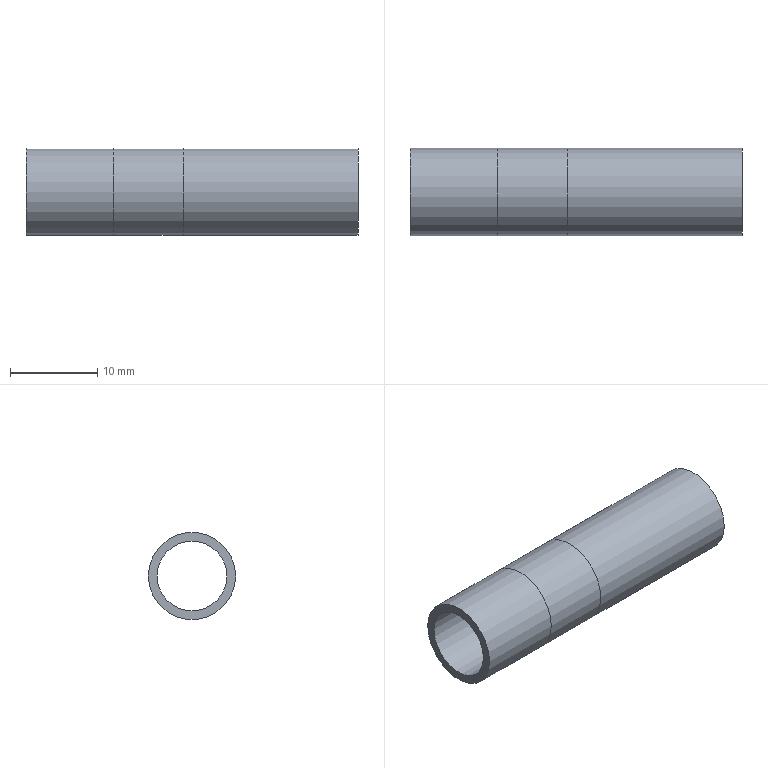Part | STEP file | 1-12.2 | 1 solid | 6 faces | box 38 x 10 x 10 mm | volume 1074 mm3 | cylinder 4 | plane 2 | commonest cylinder face diameters 10 x3 8 x1
STEP:
#1=CARTESIAN_POINT('',(0.,0.,0.));
#2=DIRECTION('',(0.,0.,1.));
#3=DIRECTION('',(1.,0.,0.));
#4=AXIS2_PLACEMENT_3D('',#1,#2,#3);
#5=CARTESIAN_POINT('',(-19.,5.,0.));
#6=VERTEX_POINT('',#5);
#7=CARTESIAN_POINT('',(-19.,0.,0.));
#8=DIRECTION('',(1.,0.,0.));
#9=DIRECTION('',(0.,1.,0.));
#10=AXIS2_PLACEMENT_3D('',#7,#8,#9);
#11=CIRCLE('',#10,5.);
#12=CARTESIAN_POINT('',(-19.,-1.34,0.));
#13=DIRECTION('',(1.,0.,0.));
#14=DIRECTION('',(0.,1.,0.));
#15=AXIS2_PLACEMENT_3D('',#12,#13,#14);
#16=PLANE('',#15);
#17=CARTESIAN_POINT('',(1.34,0.));
#18=DIRECTION('',(1.,0.));
#19=AXIS2_PLACEMENT_2D('',#17,#18);
#20=CIRCLE('',#19,5.);
#21=(GEOMETRIC_REPRESENTATION_CONTEXT(2)PARAMETRIC_REPRESENTATION_CONTEXT()REPRESENTATION_CONTEXT('',''));
#22=DEFINITIONAL_REPRESENTATION('',(#20),#21);
#23=PCURVE('',#16,#22);
#24=CARTESIAN_POINT('',(-19.,0.,0.));
#25=DIRECTION('',(1.,0.,0.));
#26=DIRECTION('',(0.,1.,0.));
#27=AXIS2_PLACEMENT_3D('',#24,#25,#26);
#28=CYLINDRICAL_SURFACE('',#27,5.);
#29=CARTESIAN_POINT('',(0.,0.));
#30=DIRECTION('',(1.,0.));
#31=VECTOR('',#30,1.);
#32=LINE('',#29,#31);
#33=(GEOMETRIC_REPRESENTATION_CONTEXT(2)PARAMETRIC_REPRESENTATION_CONTEXT()REPRESENTATION_CONTEXT('',''));
#34=DEFINITIONAL_REPRESENTATION('',(#32),#33);
#35=PCURVE('',#28,#34);
#36=SURFACE_CURVE('',#11,(#23,#35),.PCURVE_S1.);
#37=EDGE_CURVE('',#6,#6,#36,.T.);
#38=ORIENTED_EDGE('',*,*,#37,.T.);
#39=EDGE_LOOP('',(#38));
#40=FACE_BOUND('',#39,.F.);
#41=CARTESIAN_POINT('',(-19.,4.,0.));
#42=VERTEX_POINT('',#41);
#43=CARTESIAN_POINT('',(-19.,0.,0.));
#44=DIRECTION('',(-1.,0.,0.));
#45=DIRECTION('',(0.,1.,0.));
#46=AXIS2_PLACEMENT_3D('',#43,#44,#45);
#47=CIRCLE('',#46,4.);
#48=CARTESIAN_POINT('',(5.34,0.));
#49=CARTESIAN_POINT('',(5.34,-6.928));
#50=CARTESIAN_POINT('',(-0.6603,-3.464));
#51=CARTESIAN_POINT('',(-6.66,0.));
#52=CARTESIAN_POINT('',(-0.6603,3.464));
#53=CARTESIAN_POINT('',(5.34,6.928));
#54=CARTESIAN_POINT('',(5.34,0.));
#55=(BOUNDED_CURVE()B_SPLINE_CURVE(2,(#48,#49,#50,#51,#52,#53,#54),.UNSPECIFIED.,.T.,.F.)B_SPLINE_CURVE_WITH_KNOTS((1,2,2,2,2,1),(-2.094,0.,2.094,4.189,6.283,8.378),.UNSPECIFIED.)CURVE()GEOMETRIC_REPRESENTATION_ITEM()RATIONAL_B_SPLINE_CURVE((1.,0.5,1.,0.5,1.,0.5,1.))REPRESENTATION_ITEM(''));
#56=(GEOMETRIC_REPRESENTATION_CONTEXT(2)PARAMETRIC_REPRESENTATION_CONTEXT()REPRESENTATION_CONTEXT('',''));
#57=DEFINITIONAL_REPRESENTATION('',(#55),#56);
#58=PCURVE('',#16,#57);
#59=CARTESIAN_POINT('',(-19.,0.,0.));
#60=DIRECTION('',(1.,0.,0.));
#61=DIRECTION('',(0.,1.,0.));
#62=AXIS2_PLACEMENT_3D('',#59,#60,#61);
#63=CYLINDRICAL_SURFACE('',#62,4.);
#64=CARTESIAN_POINT('',(6.283,0.));
#65=DIRECTION('',(-1.,0.));
#66=VECTOR('',#65,1.);
#67=LINE('',#64,#66);
#68=(GEOMETRIC_REPRESENTATION_CONTEXT(2)PARAMETRIC_REPRESENTATION_CONTEXT()REPRESENTATION_CONTEXT('',''));
#69=DEFINITIONAL_REPRESENTATION('',(#67),#68);
#70=PCURVE('',#63,#69);
#71=SURFACE_CURVE('',#47,(#58,#70),.PCURVE_S1.);
#72=EDGE_CURVE('',#42,#42,#71,.T.);
#73=ORIENTED_EDGE('',*,*,#72,.T.);
#74=EDGE_LOOP('',(#73));
#75=FACE_BOUND('',#74,.F.);
#76=ADVANCED_FACE('',(#40,#75),#16,.F.);
#77=CARTESIAN_POINT('',(19.,5.,0.));
#78=VERTEX_POINT('',#77);
#79=CARTESIAN_POINT('',(19.,0.,0.));
#80=DIRECTION('',(1.,0.,0.));
#81=DIRECTION('',(0.,1.,0.));
#82=AXIS2_PLACEMENT_3D('',#79,#80,#81);
#83=CIRCLE('',#82,5.);
#84=CARTESIAN_POINT('',(19.,-1.34,0.));
#85=DIRECTION('',(1.,0.,0.));
#86=DIRECTION('',(0.,1.,0.));
#87=AXIS2_PLACEMENT_3D('',#84,#85,#86);
#88=PLANE('',#87);
#89=CARTESIAN_POINT('',(1.34,0.));
#90=DIRECTION('',(1.,0.));
#91=AXIS2_PLACEMENT_2D('',#89,#90);
#92=CIRCLE('',#91,5.);
#93=(GEOMETRIC_REPRESENTATION_CONTEXT(2)PARAMETRIC_REPRESENTATION_CONTEXT()REPRESENTATION_CONTEXT('',''));
#94=DEFINITIONAL_REPRESENTATION('',(#92),#93);
#95=PCURVE('',#88,#94);
#96=CARTESIAN_POINT('',(-1.,0.,0.));
#97=DIRECTION('',(1.,0.,0.));
#98=DIRECTION('',(0.,1.,0.));
#99=AXIS2_PLACEMENT_3D('',#96,#97,#98);
#100=CYLINDRICAL_SURFACE('',#99,5.);
#101=CARTESIAN_POINT('',(0.,20.));
#102=DIRECTION('',(1.,0.));
#103=VECTOR('',#102,1.);
#104=LINE('',#101,#103);
#105=(GEOMETRIC_REPRESENTATION_CONTEXT(2)PARAMETRIC_REPRESENTATION_CONTEXT()REPRESENTATION_CONTEXT('',''));
#106=DEFINITIONAL_REPRESENTATION('',(#104),#105);
#107=PCURVE('',#100,#106);
#108=SURFACE_CURVE('',#83,(#95,#107),.PCURVE_S1.);
#109=EDGE_CURVE('',#78,#78,#108,.T.);
#110=ORIENTED_EDGE('',*,*,#109,.T.);
#111=EDGE_LOOP('',(#110));
#112=FACE_BOUND('',#111,.T.);
#113=CARTESIAN_POINT('',(19.,4.,0.));
#114=VERTEX_POINT('',#113);
#115=CARTESIAN_POINT('',(19.,0.,0.));
#116=DIRECTION('',(-1.,0.,0.));
#117=DIRECTION('',(0.,1.,0.));
#118=AXIS2_PLACEMENT_3D('',#115,#116,#117);
#119=CIRCLE('',#118,4.);
#120=CARTESIAN_POINT('',(5.34,0.));
#121=CARTESIAN_POINT('',(5.34,-6.928));
#122=CARTESIAN_POINT('',(-0.6603,-3.464));
#123=CARTESIAN_POINT('',(-6.66,0.));
#124=CARTESIAN_POINT('',(-0.6603,3.464));
#125=CARTESIAN_POINT('',(5.34,6.928));
#126=CARTESIAN_POINT('',(5.34,0.));
#127=(BOUNDED_CURVE()B_SPLINE_CURVE(2,(#120,#121,#122,#123,#124,#125,#126),.UNSPECIFIED.,.T.,.F.)B_SPLINE_CURVE_WITH_KNOTS((1,2,2,2,2,1),(-2.094,0.,2.094,4.189,6.283,8.378),.UNSPECIFIED.)CURVE()GEOMETRIC_REPRESENTATION_ITEM()RATIONAL_B_SPLINE_CURVE((1.,0.5,1.,0.5,1.,0.5,1.))REPRESENTATION_ITEM(''));
#128=(GEOMETRIC_REPRESENTATION_CONTEXT(2)PARAMETRIC_REPRESENTATION_CONTEXT()REPRESENTATION_CONTEXT('',''));
#129=DEFINITIONAL_REPRESENTATION('',(#127),#128);
#130=PCURVE('',#88,#129);
#131=CARTESIAN_POINT('',(6.283,38.));
#132=DIRECTION('',(-1.,0.));
#133=VECTOR('',#132,1.);
#134=LINE('',#131,#133);
#135=(GEOMETRIC_REPRESENTATION_CONTEXT(2)PARAMETRIC_REPRESENTATION_CONTEXT()REPRESENTATION_CONTEXT('',''));
#136=DEFINITIONAL_REPRESENTATION('',(#134),#135);
#137=PCURVE('',#63,#136);
#138=SURFACE_CURVE('',#119,(#130,#137),.PCURVE_S1.);
#139=EDGE_CURVE('',#114,#114,#138,.T.);
#140=ORIENTED_EDGE('',*,*,#139,.T.);
#141=EDGE_LOOP('',(#140));
#142=FACE_BOUND('',#141,.T.);
#143=ADVANCED_FACE('',(#112,#142),#88,.T.);
#144=CARTESIAN_POINT('',(-19.,4.,0.));
#145=DIRECTION('',(1.,0.,0.));
#146=VECTOR('',#145,1.);
#147=LINE('',#144,#146);
#148=CARTESIAN_POINT('',(6.283,0.));
#149=DIRECTION('',(0.,1.));
#150=VECTOR('',#149,1.);
#151=LINE('',#148,#150);
#152=(GEOMETRIC_REPRESENTATION_CONTEXT(2)PARAMETRIC_REPRESENTATION_CONTEXT()REPRESENTATION_CONTEXT('',''));
#153=DEFINITIONAL_REPRESENTATION('',(#151),#152);
#154=PCURVE('',#63,#153);
#155=CARTESIAN_POINT('',(0.,0.));
#156=DIRECTION('',(0.,1.));
#157=VECTOR('',#156,1.);
#158=LINE('',#155,#157);
#159=(GEOMETRIC_REPRESENTATION_CONTEXT(2)PARAMETRIC_REPRESENTATION_CONTEXT()REPRESENTATION_CONTEXT('',''));
#160=DEFINITIONAL_REPRESENTATION('',(#158),#159);
#161=PCURVE('',#63,#160);
#162=SEAM_CURVE('',#147,(#154,#161),.PCURVE_S1.);
#163=EDGE_CURVE('',#42,#114,#162,.T.);
#164=ORIENTED_EDGE('',*,*,#163,.T.);
#165=ORIENTED_EDGE('',*,*,#139,.T.);
#166=ORIENTED_EDGE('',*,*,#163,.F.);
#167=ORIENTED_EDGE('',*,*,#72,.F.);
#168=EDGE_LOOP('',(#164,#165,#166,#167));
#169=FACE_BOUND('',#168,.F.);
#170=ADVANCED_FACE('',(#169),#63,.F.);
#171=ORIENTED_EDGE('',*,*,#37,.T.);
#172=CARTESIAN_POINT('',(-9.,5.,0.));
#173=VERTEX_POINT('',#172);
#174=CARTESIAN_POINT('',(-19.,5.,0.));
#175=DIRECTION('',(1.,0.,0.));
#176=VECTOR('',#175,1.);
#177=LINE('',#174,#176);
#178=CARTESIAN_POINT('',(6.283,0.));
#179=DIRECTION('',(0.,1.));
#180=VECTOR('',#179,1.);
#181=LINE('',#178,#180);
#182=(GEOMETRIC_REPRESENTATION_CONTEXT(2)PARAMETRIC_REPRESENTATION_CONTEXT()REPRESENTATION_CONTEXT('',''));
#183=DEFINITIONAL_REPRESENTATION('',(#181),#182);
#184=PCURVE('',#28,#183);
#185=CARTESIAN_POINT('',(0.,0.));
#186=DIRECTION('',(0.,1.));
#187=VECTOR('',#186,1.);
#188=LINE('',#185,#187);
#189=(GEOMETRIC_REPRESENTATION_CONTEXT(2)PARAMETRIC_REPRESENTATION_CONTEXT()REPRESENTATION_CONTEXT('',''));
#190=DEFINITIONAL_REPRESENTATION('',(#188),#189);
#191=PCURVE('',#28,#190);
#192=SEAM_CURVE('',#177,(#184,#191),.PCURVE_S1.);
#193=EDGE_CURVE('',#6,#173,#192,.T.);
#194=ORIENTED_EDGE('',*,*,#193,.T.);
#195=CARTESIAN_POINT('',(-9.,0.,0.));
#196=DIRECTION('',(1.,0.,0.));
#197=DIRECTION('',(0.,1.,0.));
#198=AXIS2_PLACEMENT_3D('',#195,#196,#197);
#199=CIRCLE('',#198,5.);
#200=CARTESIAN_POINT('',(0.,10.));
#201=DIRECTION('',(1.,0.));
#202=VECTOR('',#201,1.);
#203=LINE('',#200,#202);
#204=(GEOMETRIC_REPRESENTATION_CONTEXT(2)PARAMETRIC_REPRESENTATION_CONTEXT()REPRESENTATION_CONTEXT('',''));
#205=DEFINITIONAL_REPRESENTATION('',(#203),#204);
#206=PCURVE('',#28,#205);
#207=CARTESIAN_POINT('',(-19.,0.,0.));
#208=DIRECTION('',(1.,0.,0.));
#209=DIRECTION('',(0.,1.,0.));
#210=AXIS2_PLACEMENT_3D('',#207,#208,#209);
#211=CYLINDRICAL_SURFACE('',#210,5.);
#212=CARTESIAN_POINT('',(0.,10.));
#213=DIRECTION('',(1.,0.));
#214=VECTOR('',#213,1.);
#215=LINE('',#212,#214);
#216=(GEOMETRIC_REPRESENTATION_CONTEXT(2)PARAMETRIC_REPRESENTATION_CONTEXT()REPRESENTATION_CONTEXT('',''));
#217=DEFINITIONAL_REPRESENTATION('',(#215),#216);
#218=PCURVE('',#211,#217);
#219=SURFACE_CURVE('',#199,(#206,#218),.PCURVE_S1.);
#220=EDGE_CURVE('',#173,#173,#219,.T.);
#221=ORIENTED_EDGE('',*,*,#220,.F.);
#222=ORIENTED_EDGE('',*,*,#193,.F.);
#223=EDGE_LOOP('',(#171,#194,#221,#222));
#224=FACE_BOUND('',#223,.T.);
#225=ADVANCED_FACE('',(#224),#28,.T.);
#226=ORIENTED_EDGE('',*,*,#220,.T.);
#227=CARTESIAN_POINT('',(-1.,5.,0.));
#228=VERTEX_POINT('',#227);
#229=CARTESIAN_POINT('',(-9.,5.,0.));
#230=DIRECTION('',(1.,0.,0.));
#231=VECTOR('',#230,1.);
#232=LINE('',#229,#231);
#233=CARTESIAN_POINT('',(6.283,10.));
#234=DIRECTION('',(0.,1.));
#235=VECTOR('',#234,1.);
#236=LINE('',#233,#235);
#237=(GEOMETRIC_REPRESENTATION_CONTEXT(2)PARAMETRIC_REPRESENTATION_CONTEXT()REPRESENTATION_CONTEXT('',''));
#238=DEFINITIONAL_REPRESENTATION('',(#236),#237);
#239=PCURVE('',#211,#238);
#240=CARTESIAN_POINT('',(0.,10.));
#241=DIRECTION('',(0.,1.));
#242=VECTOR('',#241,1.);
#243=LINE('',#240,#242);
#244=(GEOMETRIC_REPRESENTATION_CONTEXT(2)PARAMETRIC_REPRESENTATION_CONTEXT()REPRESENTATION_CONTEXT('',''));
#245=DEFINITIONAL_REPRESENTATION('',(#243),#244);
#246=PCURVE('',#211,#245);
#247=SEAM_CURVE('',#232,(#239,#246),.PCURVE_S1.);
#248=EDGE_CURVE('',#173,#228,#247,.T.);
#249=ORIENTED_EDGE('',*,*,#248,.T.);
#250=CARTESIAN_POINT('',(-1.,0.,0.));
#251=DIRECTION('',(1.,0.,0.));
#252=DIRECTION('',(0.,1.,0.));
#253=AXIS2_PLACEMENT_3D('',#250,#251,#252);
#254=CIRCLE('',#253,5.);
#255=CARTESIAN_POINT('',(0.,18.));
#256=DIRECTION('',(1.,0.));
#257=VECTOR('',#256,1.);
#258=LINE('',#255,#257);
#259=(GEOMETRIC_REPRESENTATION_CONTEXT(2)PARAMETRIC_REPRESENTATION_CONTEXT()REPRESENTATION_CONTEXT('',''));
#260=DEFINITIONAL_REPRESENTATION('',(#258),#259);
#261=PCURVE('',#211,#260);
#262=CARTESIAN_POINT('',(0.,0.));
#263=DIRECTION('',(1.,0.));
#264=VECTOR('',#263,1.);
#265=LINE('',#262,#264);
#266=(GEOMETRIC_REPRESENTATION_CONTEXT(2)PARAMETRIC_REPRESENTATION_CONTEXT()REPRESENTATION_CONTEXT('',''));
#267=DEFINITIONAL_REPRESENTATION('',(#265),#266);
#268=PCURVE('',#100,#267);
#269=SURFACE_CURVE('',#254,(#261,#268),.PCURVE_S1.);
#270=EDGE_CURVE('',#228,#228,#269,.T.);
#271=ORIENTED_EDGE('',*,*,#270,.F.);
#272=ORIENTED_EDGE('',*,*,#248,.F.);
#273=EDGE_LOOP('',(#226,#249,#271,#272));
#274=FACE_BOUND('',#273,.T.);
#275=ADVANCED_FACE('',(#274),#211,.T.);
#276=ORIENTED_EDGE('',*,*,#109,.F.);
#277=CARTESIAN_POINT('',(-1.,5.,0.));
#278=DIRECTION('',(1.,0.,0.));
#279=VECTOR('',#278,1.);
#280=LINE('',#277,#279);
#281=CARTESIAN_POINT('',(0.,0.));
#282=DIRECTION('',(0.,1.));
#283=VECTOR('',#282,1.);
#284=LINE('',#281,#283);
#285=(GEOMETRIC_REPRESENTATION_CONTEXT(2)PARAMETRIC_REPRESENTATION_CONTEXT()REPRESENTATION_CONTEXT('',''));
#286=DEFINITIONAL_REPRESENTATION('',(#284),#285);
#287=PCURVE('',#100,#286);
#288=CARTESIAN_POINT('',(6.283,0.));
#289=DIRECTION('',(0.,1.));
#290=VECTOR('',#289,1.);
#291=LINE('',#288,#290);
#292=(GEOMETRIC_REPRESENTATION_CONTEXT(2)PARAMETRIC_REPRESENTATION_CONTEXT()REPRESENTATION_CONTEXT('',''));
#293=DEFINITIONAL_REPRESENTATION('',(#291),#292);
#294=PCURVE('',#100,#293);
#295=SEAM_CURVE('',#280,(#287,#294),.PCURVE_S1.);
#296=EDGE_CURVE('',#228,#78,#295,.T.);
#297=ORIENTED_EDGE('',*,*,#296,.F.);
#298=ORIENTED_EDGE('',*,*,#270,.T.);
#299=ORIENTED_EDGE('',*,*,#296,.T.);
#300=EDGE_LOOP('',(#276,#297,#298,#299));
#301=FACE_BOUND('',#300,.T.);
#302=ADVANCED_FACE('',(#301),#100,.T.);
#303=CLOSED_SHELL('',(#76,#143,#170,#225,#275,#302));
#304=MANIFOLD_SOLID_BREP('',#303);
#305=(LENGTH_UNIT()NAMED_UNIT(*)SI_UNIT(.MILLI.,.METRE.));
#306=UNCERTAINTY_MEASURE_WITH_UNIT(LENGTH_MEASURE(0.0000001),#305,'','');
#307=(NAMED_UNIT(*)PLANE_ANGLE_UNIT()SI_UNIT($,.RADIAN.));
#308=(NAMED_UNIT(*)SI_UNIT($,.STERADIAN.)SOLID_ANGLE_UNIT());
#309=(GEOMETRIC_REPRESENTATION_CONTEXT(3)GLOBAL_UNCERTAINTY_ASSIGNED_CONTEXT((#306))GLOBAL_UNIT_ASSIGNED_CONTEXT((#305,#307,#308))REPRESENTATION_CONTEXT('',''));
#310=ADVANCED_BREP_SHAPE_REPRESENTATION('',(#4,#304),#309);